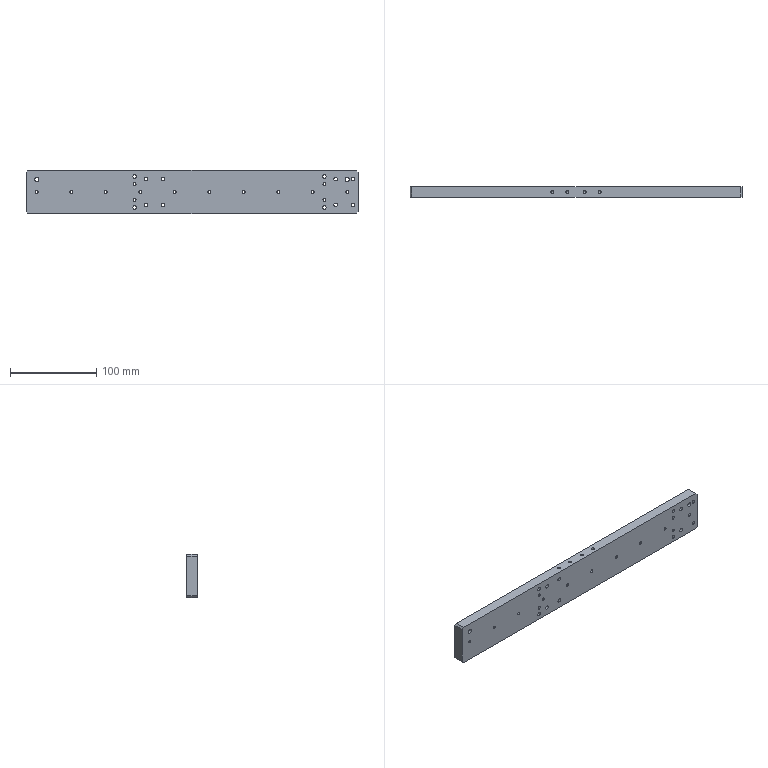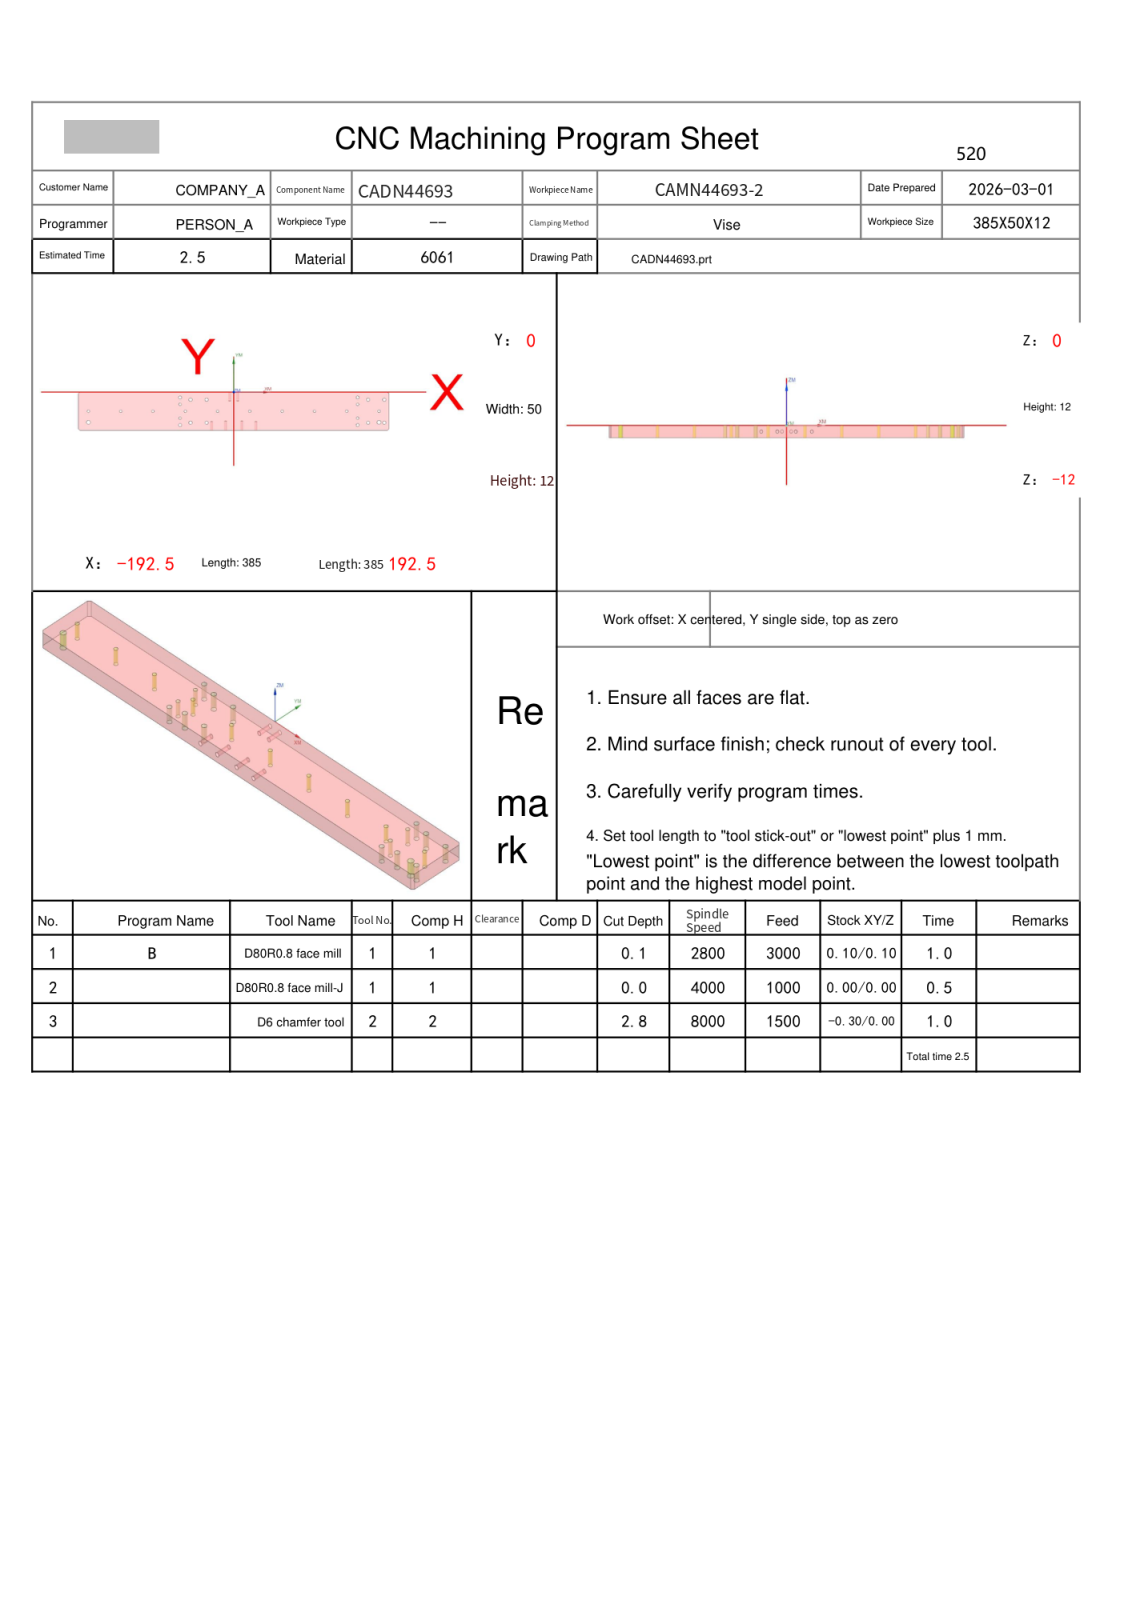NC program | NX | posted by the shop | part box 385 x 12 x 50 mm
Whole program:
%
O0001
(Machine time: 3.02 MIN)
(===Total Tool:2===)
(T1=D80R0.8 face mill D=80.  R=0.8  D-  H01 Z=-0.   )
(T2=D6 chamfer tool   D=6.   R=0.   D-  H02 Z=-2.8  )
G80 G90 G17 G49 G40
G91 G28 Z0
M01
N1 T01 M06
(D80R0.8 face mill  D=80. R=0.8 H=01 ce=0.10 di=0.10)
G00 G90 G54 X244.597 Y-25. M03 S2800
G43 H01 Z50.
M08
Z4.02
G01 Z2.02 F3000.
X232.597
X-232.597
X-244.597
Z4.02
G00 X244.597
Z3.54
G01 Z1.54
X232.597
X-232.597
X-244.597
Z3.54
G00 X244.597
Z3.06
G01 Z1.06
X232.597
X-232.597
X-244.597
Z3.06
G00 X244.597
Z2.58
G01 Z.58
X232.597
X-232.597
X-244.597
Z2.58
G00 Z50.
X244.597
Z2.1
G01 Z.1
X232.597
X-232.597
X-244.597
Z2.1
G00 Z50.
G91 G28 Z0.0
M05
M09
G91 G28 Z0.0
M01
N2 T01 M06
(D80R0.8 face mill-J  D=80. R=0.8 H=01 ce=0.00 di=0.00)
G00 G90 G54 X244.499 Y-25. M03 S4000
G43 H01 Z50.
M08
Z2.
G01 Z0.0 F1000.
X232.499
X-232.499
X-244.499
Z2.
G00 Z50.
G91 G28 Z0.0
M05
M09
G91 G28 Z0.0
M01
N3 T02 M06
(D6 chamfer tool  D=6. R=0. H=02 ce=0.00 di=0.00)
G00 G90 G54 X-180. Y-25. M03 S8000
G43 H02 Z50.
M08
G98 G81 X-180. Y-25. Z-2.2 R3. F1000.
X-140.
X-100.
X-66.5 Y-34.
Y-16.
X-60. Y-25.
X-20.
X20.
X60.
X100.
X140.
X153.5 Y-34.
Y-16.
X180. Y-25.
G80
G00 Z50.
G00 G90 X-66.5 Y-7. M03 S8000
Z50.
G98 G81 X-66.5 Y-7. Z-2.3 R3. F1000.
Y-43.
X153.5
Y-7.
G80
G00 Z50.
G00 G90 X180. Y-39.5 M03 S8000
Z50.
G98 G81 X180. Y-39.5 Z-2.8 R3. F1000.
X-180.
G80
G00 Z50.
G00 G90 X-33.5 Y-10. M03 S8000
Z50.
G98 G81 X-33.5 Y-10. Z-2.7 R3. F1000.
X-53.5
Y-40.
X-33.5
X166.5
X186.5
Y-10.
X166.5
G80
G00 Z50.
G00 G90 X181.546 Y.7 M03 S7000
Z50.
Z2.5
G01 X190.376 Z-.714 F1500.
X190.453 Z-.742
X190.66 Y.662 Z-.819
X190.855 Y.581 Z-.895
X191.028 Y.462 Z-.972
X191.083 Y.407 Z-1.
X192.907 Y-1.417
G02 X193.2 Y-2.124 I-.707 J-.707
G01 Y-47.876
G02 X192.907 Y-48.583 I-1. J0.0
G01 X191.083 Y-50.407
G02 X190.376 Y-50.7 I-.707 J.707
G01 X-190.376
G02 X-191.083 Y-50.407 I0.0 J1.
G01 X-192.907 Y-48.583
G02 X-193.2 Y-47.876 I.707 J.707
G01 Y-2.124
G02 X-192.907 Y-1.417 I1. J0.0
G01 X-191.083 Y.407
G02 X-190.376 Y.7 I.707 J-.707
G01 X190.376
G02 X191.083 Y.407 I0.0 J-1.
G01 X191.436 Y.054
Z1.5
G00 Z50.
M05
M09
G91 G28 Z0.0
G91 G28 Y0.0
M30
%